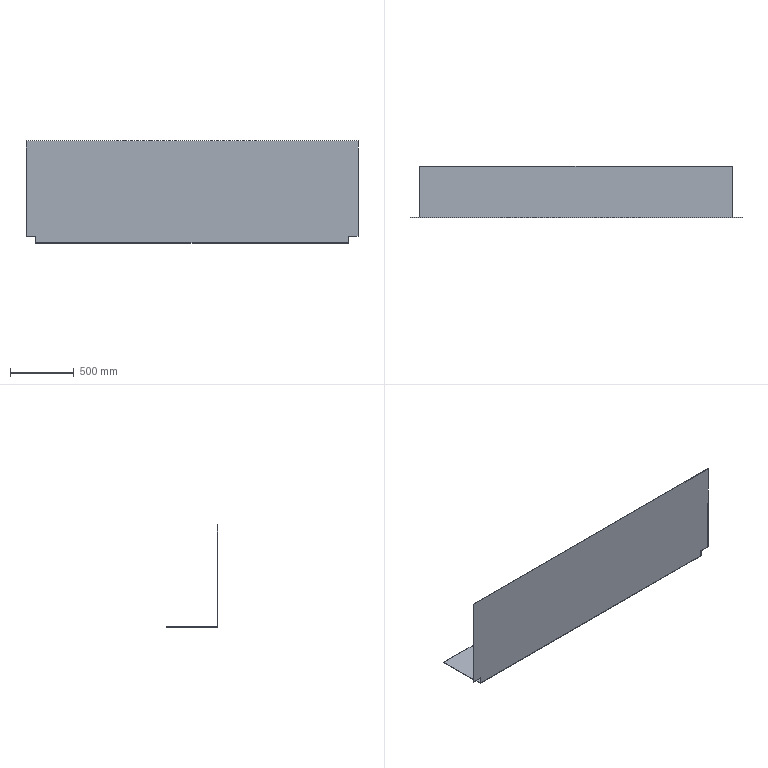Part | STEP file | E3-花纹Plate折弯3 | 1 solid | 14 faces | box 2596 x 403 x 798 mm | volume 9110634 mm3 | plane 12 | cylinder 2 | commonest cylinder face diameters 2 x1 8 x1
STEP:
#1=CARTESIAN_POINT('',(0.,0.,0.));
#2=DIRECTION('',(0.,0.,1.));
#3=DIRECTION('',(1.,0.,0.));
#4=AXIS2_PLACEMENT_3D('',#1,#2,#3);
#5=CARTESIAN_POINT('',(2596.,0.,-746.));
#6=VERTEX_POINT('',#5);
#7=CARTESIAN_POINT('',(2596.,3.,-746.));
#8=VERTEX_POINT('',#7);
#9=CARTESIAN_POINT('',(2596.,3.,-746.));
#10=DIRECTION('',(0.,1.,0.));
#11=VECTOR('',#10,1.);
#12=LINE('',#9,#11);
#13=CARTESIAN_POINT('',(2596.,3.,0.));
#14=DIRECTION('',(1.,0.,0.));
#15=DIRECTION('',(0.,0.,1.));
#16=AXIS2_PLACEMENT_3D('',#13,#14,#15);
#17=PLANE('',#16);
#18=CARTESIAN_POINT('',(-746.,0.));
#19=DIRECTION('',(0.,-1.));
#20=VECTOR('',#19,1.);
#21=LINE('',#18,#20);
#22=(GEOMETRIC_REPRESENTATION_CONTEXT(2)PARAMETRIC_REPRESENTATION_CONTEXT()REPRESENTATION_CONTEXT('',''));
#23=DEFINITIONAL_REPRESENTATION('',(#21),#22);
#24=PCURVE('',#17,#23);
#25=CARTESIAN_POINT('',(2518.,-497.,-746.));
#26=DIRECTION('',(0.,0.,1.));
#27=DIRECTION('',(-1.,0.,0.));
#28=AXIS2_PLACEMENT_3D('',#25,#26,#27);
#29=PLANE('',#28);
#30=CARTESIAN_POINT('',(-78.,-500.));
#31=DIRECTION('',(0.,-1.));
#32=VECTOR('',#31,1.);
#33=LINE('',#30,#32);
#34=(GEOMETRIC_REPRESENTATION_CONTEXT(2)PARAMETRIC_REPRESENTATION_CONTEXT()REPRESENTATION_CONTEXT('',''));
#35=DEFINITIONAL_REPRESENTATION('',(#33),#34);
#36=PCURVE('',#29,#35);
#37=SURFACE_CURVE('',#12,(#24,#36),.PCURVE_S1.);
#38=EDGE_CURVE('',#6,#8,#37,.T.);
#39=ORIENTED_EDGE('',*,*,#38,.T.);
#40=CARTESIAN_POINT('',(2596.,3.,0.));
#41=VERTEX_POINT('',#40);
#42=CARTESIAN_POINT('',(2596.,3.,0.));
#43=DIRECTION('',(0.,0.,1.));
#44=VECTOR('',#43,1.);
#45=LINE('',#42,#44);
#46=CARTESIAN_POINT('',(0.,0.));
#47=DIRECTION('',(1.,0.));
#48=VECTOR('',#47,1.);
#49=LINE('',#46,#48);
#50=(GEOMETRIC_REPRESENTATION_CONTEXT(2)PARAMETRIC_REPRESENTATION_CONTEXT()REPRESENTATION_CONTEXT('',''));
#51=DEFINITIONAL_REPRESENTATION('',(#49),#50);
#52=PCURVE('',#17,#51);
#53=CARTESIAN_POINT('',(0.,3.,0.));
#54=DIRECTION('',(0.,1.,0.));
#55=DIRECTION('',(0.,0.,-1.));
#56=AXIS2_PLACEMENT_3D('',#53,#54,#55);
#57=PLANE('',#56);
#58=CARTESIAN_POINT('',(0.,-2596.));
#59=DIRECTION('',(-1.,0.));
#60=VECTOR('',#59,1.);
#61=LINE('',#58,#60);
#62=(GEOMETRIC_REPRESENTATION_CONTEXT(2)PARAMETRIC_REPRESENTATION_CONTEXT()REPRESENTATION_CONTEXT('',''));
#63=DEFINITIONAL_REPRESENTATION('',(#61),#62);
#64=PCURVE('',#57,#63);
#65=SURFACE_CURVE('',#45,(#52,#64),.PCURVE_S1.);
#66=EDGE_CURVE('',#8,#41,#65,.T.);
#67=ORIENTED_EDGE('',*,*,#66,.T.);
#68=CARTESIAN_POINT('',(2596.,0.,0.));
#69=VERTEX_POINT('',#68);
#70=CARTESIAN_POINT('',(2596.,3.,0.));
#71=DIRECTION('',(0.,1.,0.));
#72=VECTOR('',#71,1.);
#73=LINE('',#70,#72);
#74=CARTESIAN_POINT('',(0.,0.));
#75=DIRECTION('',(0.,-1.));
#76=VECTOR('',#75,1.);
#77=LINE('',#74,#76);
#78=(GEOMETRIC_REPRESENTATION_CONTEXT(2)PARAMETRIC_REPRESENTATION_CONTEXT()REPRESENTATION_CONTEXT('',''));
#79=DEFINITIONAL_REPRESENTATION('',(#77),#78);
#80=PCURVE('',#17,#79);
#81=CARTESIAN_POINT('',(0.,3.,0.));
#82=DIRECTION('',(0.,0.,1.));
#83=DIRECTION('',(-1.,0.,0.));
#84=AXIS2_PLACEMENT_3D('',#81,#82,#83);
#85=PLANE('',#84);
#86=CARTESIAN_POINT('',(-2596.,0.));
#87=DIRECTION('',(0.,-1.));
#88=VECTOR('',#87,1.);
#89=LINE('',#86,#88);
#90=(GEOMETRIC_REPRESENTATION_CONTEXT(2)PARAMETRIC_REPRESENTATION_CONTEXT()REPRESENTATION_CONTEXT('',''));
#91=DEFINITIONAL_REPRESENTATION('',(#89),#90);
#92=PCURVE('',#85,#91);
#93=SURFACE_CURVE('',#73,(#80,#92),.PCURVE_S1.);
#94=EDGE_CURVE('',#69,#41,#93,.T.);
#95=ORIENTED_EDGE('',*,*,#94,.F.);
#96=CARTESIAN_POINT('',(2596.,0.,0.));
#97=DIRECTION('',(0.,0.,1.));
#98=VECTOR('',#97,1.);
#99=LINE('',#96,#98);
#100=CARTESIAN_POINT('',(0.,3.));
#101=DIRECTION('',(1.,0.));
#102=VECTOR('',#101,1.);
#103=LINE('',#100,#102);
#104=(GEOMETRIC_REPRESENTATION_CONTEXT(2)PARAMETRIC_REPRESENTATION_CONTEXT()REPRESENTATION_CONTEXT('',''));
#105=DEFINITIONAL_REPRESENTATION('',(#103),#104);
#106=PCURVE('',#17,#105);
#107=CARTESIAN_POINT('',(0.,0.,0.));
#108=DIRECTION('',(0.,1.,0.));
#109=DIRECTION('',(0.,0.,-1.));
#110=AXIS2_PLACEMENT_3D('',#107,#108,#109);
#111=PLANE('',#110);
#112=CARTESIAN_POINT('',(0.,-2596.));
#113=DIRECTION('',(-1.,0.));
#114=VECTOR('',#113,1.);
#115=LINE('',#112,#114);
#116=(GEOMETRIC_REPRESENTATION_CONTEXT(2)PARAMETRIC_REPRESENTATION_CONTEXT()REPRESENTATION_CONTEXT('',''));
#117=DEFINITIONAL_REPRESENTATION('',(#115),#116);
#118=PCURVE('',#111,#117);
#119=SURFACE_CURVE('',#99,(#106,#118),.PCURVE_S1.);
#120=EDGE_CURVE('',#6,#69,#119,.T.);
#121=ORIENTED_EDGE('',*,*,#120,.F.);
#122=EDGE_LOOP('',(#39,#67,#95,#121));
#123=FACE_BOUND('',#122,.T.);
#124=ADVANCED_FACE('',(#123),#17,.T.);
#125=CARTESIAN_POINT('',(2518.,3.,-746.));
#126=VERTEX_POINT('',#125);
#127=CARTESIAN_POINT('',(2518.,3.,-794.));
#128=VERTEX_POINT('',#127);
#129=CARTESIAN_POINT('',(2518.,3.,0.));
#130=DIRECTION('',(0.,0.,-1.));
#131=VECTOR('',#130,1.);
#132=LINE('',#129,#131);
#133=CARTESIAN_POINT('',(0.,-2518.));
#134=DIRECTION('',(1.,0.));
#135=VECTOR('',#134,1.);
#136=LINE('',#133,#135);
#137=(GEOMETRIC_REPRESENTATION_CONTEXT(2)PARAMETRIC_REPRESENTATION_CONTEXT()REPRESENTATION_CONTEXT('',''));
#138=DEFINITIONAL_REPRESENTATION('',(#136),#137);
#139=PCURVE('',#57,#138);
#140=CARTESIAN_POINT('',(2518.,-497.,-798.));
#141=DIRECTION('',(-1.,0.,0.));
#142=DIRECTION('',(0.,0.,-1.));
#143=AXIS2_PLACEMENT_3D('',#140,#141,#142);
#144=PLANE('',#143);
#145=CARTESIAN_POINT('',(-798.,-500.));
#146=DIRECTION('',(1.,0.));
#147=VECTOR('',#146,1.);
#148=LINE('',#145,#147);
#149=(GEOMETRIC_REPRESENTATION_CONTEXT(2)PARAMETRIC_REPRESENTATION_CONTEXT()REPRESENTATION_CONTEXT('',''));
#150=DEFINITIONAL_REPRESENTATION('',(#148),#149);
#151=PCURVE('',#144,#150);
#152=SURFACE_CURVE('',#132,(#139,#151),.PCURVE_S1.);
#153=EDGE_CURVE('',#126,#128,#152,.T.);
#154=ORIENTED_EDGE('',*,*,#153,.T.);
#155=CARTESIAN_POINT('',(78.,3.,-794.));
#156=VERTEX_POINT('',#155);
#157=CARTESIAN_POINT('',(2596.,3.,-794.));
#158=DIRECTION('',(-1.,0.,0.));
#159=VECTOR('',#158,1.);
#160=LINE('',#157,#159);
#161=CARTESIAN_POINT('',(794.,-2596.));
#162=DIRECTION('',(0.,1.));
#163=VECTOR('',#162,1.);
#164=LINE('',#161,#163);
#165=(GEOMETRIC_REPRESENTATION_CONTEXT(2)PARAMETRIC_REPRESENTATION_CONTEXT()REPRESENTATION_CONTEXT('',''));
#166=DEFINITIONAL_REPRESENTATION('',(#164),#165);
#167=PCURVE('',#57,#166);
#168=CARTESIAN_POINT('',(2596.,4.,-794.));
#169=DIRECTION('',(1.,0.,0.));
#170=DIRECTION('',(0.,0.,-1.));
#171=AXIS2_PLACEMENT_3D('',#168,#169,#170);
#172=CYLINDRICAL_SURFACE('',#171,1.);
#173=CARTESIAN_POINT('',(4.712,0.));
#174=DIRECTION('',(0.,-1.));
#175=VECTOR('',#174,1.);
#176=LINE('',#173,#175);
#177=(GEOMETRIC_REPRESENTATION_CONTEXT(2)PARAMETRIC_REPRESENTATION_CONTEXT()REPRESENTATION_CONTEXT('',''));
#178=DEFINITIONAL_REPRESENTATION('',(#176),#177);
#179=PCURVE('',#172,#178);
#180=SURFACE_CURVE('',#160,(#167,#179),.PCURVE_S1.);
#181=EDGE_CURVE('',#128,#156,#180,.T.);
#182=ORIENTED_EDGE('',*,*,#181,.T.);
#183=CARTESIAN_POINT('',(78.,3.,-746.));
#184=VERTEX_POINT('',#183);
#185=CARTESIAN_POINT('',(78.,3.,0.));
#186=DIRECTION('',(0.,0.,1.));
#187=VECTOR('',#186,1.);
#188=LINE('',#185,#187);
#189=CARTESIAN_POINT('',(0.,-78.));
#190=DIRECTION('',(-1.,0.));
#191=VECTOR('',#190,1.);
#192=LINE('',#189,#191);
#193=(GEOMETRIC_REPRESENTATION_CONTEXT(2)PARAMETRIC_REPRESENTATION_CONTEXT()REPRESENTATION_CONTEXT('',''));
#194=DEFINITIONAL_REPRESENTATION('',(#192),#193);
#195=PCURVE('',#57,#194);
#196=CARTESIAN_POINT('',(78.,-497.,-798.));
#197=DIRECTION('',(1.,0.,0.));
#198=DIRECTION('',(0.,0.,1.));
#199=AXIS2_PLACEMENT_3D('',#196,#197,#198);
#200=PLANE('',#199);
#201=CARTESIAN_POINT('',(798.,-500.));
#202=DIRECTION('',(1.,0.));
#203=VECTOR('',#202,1.);
#204=LINE('',#201,#203);
#205=(GEOMETRIC_REPRESENTATION_CONTEXT(2)PARAMETRIC_REPRESENTATION_CONTEXT()REPRESENTATION_CONTEXT('',''));
#206=DEFINITIONAL_REPRESENTATION('',(#204),#205);
#207=PCURVE('',#200,#206);
#208=SURFACE_CURVE('',#188,(#195,#207),.PCURVE_S1.);
#209=EDGE_CURVE('',#156,#184,#208,.T.);
#210=ORIENTED_EDGE('',*,*,#209,.T.);
#211=CARTESIAN_POINT('',(0.,3.,-746.));
#212=VERTEX_POINT('',#211);
#213=CARTESIAN_POINT('',(0.,3.,-746.));
#214=DIRECTION('',(-1.,0.,0.));
#215=VECTOR('',#214,1.);
#216=LINE('',#213,#215);
#217=CARTESIAN_POINT('',(746.,0.));
#218=DIRECTION('',(0.,1.));
#219=VECTOR('',#218,1.);
#220=LINE('',#217,#219);
#221=(GEOMETRIC_REPRESENTATION_CONTEXT(2)PARAMETRIC_REPRESENTATION_CONTEXT()REPRESENTATION_CONTEXT('',''));
#222=DEFINITIONAL_REPRESENTATION('',(#220),#221);
#223=PCURVE('',#57,#222);
#224=CARTESIAN_POINT('',(-82.,-497.,-746.));
#225=DIRECTION('',(0.,0.,1.));
#226=DIRECTION('',(-1.,0.,0.));
#227=AXIS2_PLACEMENT_3D('',#224,#225,#226);
#228=PLANE('',#227);
#229=CARTESIAN_POINT('',(-82.,-500.));
#230=DIRECTION('',(1.,0.));
#231=VECTOR('',#230,1.);
#232=LINE('',#229,#231);
#233=(GEOMETRIC_REPRESENTATION_CONTEXT(2)PARAMETRIC_REPRESENTATION_CONTEXT()REPRESENTATION_CONTEXT('',''));
#234=DEFINITIONAL_REPRESENTATION('',(#232),#233);
#235=PCURVE('',#228,#234);
#236=SURFACE_CURVE('',#216,(#223,#235),.PCURVE_S1.);
#237=EDGE_CURVE('',#184,#212,#236,.T.);
#238=ORIENTED_EDGE('',*,*,#237,.T.);
#239=CARTESIAN_POINT('',(0.,3.,0.));
#240=VERTEX_POINT('',#239);
#241=CARTESIAN_POINT('',(0.,3.,0.));
#242=DIRECTION('',(0.,0.,-1.));
#243=VECTOR('',#242,1.);
#244=LINE('',#241,#243);
#245=CARTESIAN_POINT('',(0.,0.));
#246=DIRECTION('',(1.,0.));
#247=VECTOR('',#246,1.);
#248=LINE('',#245,#247);
#249=(GEOMETRIC_REPRESENTATION_CONTEXT(2)PARAMETRIC_REPRESENTATION_CONTEXT()REPRESENTATION_CONTEXT('',''));
#250=DEFINITIONAL_REPRESENTATION('',(#248),#249);
#251=PCURVE('',#57,#250);
#252=CARTESIAN_POINT('',(0.,3.,0.));
#253=DIRECTION('',(-1.,0.,0.));
#254=DIRECTION('',(0.,0.,-1.));
#255=AXIS2_PLACEMENT_3D('',#252,#253,#254);
#256=PLANE('',#255);
#257=CARTESIAN_POINT('',(0.,0.));
#258=DIRECTION('',(1.,0.));
#259=VECTOR('',#258,1.);
#260=LINE('',#257,#259);
#261=(GEOMETRIC_REPRESENTATION_CONTEXT(2)PARAMETRIC_REPRESENTATION_CONTEXT()REPRESENTATION_CONTEXT('',''));
#262=DEFINITIONAL_REPRESENTATION('',(#260),#261);
#263=PCURVE('',#256,#262);
#264=SURFACE_CURVE('',#244,(#251,#263),.PCURVE_S1.);
#265=EDGE_CURVE('',#240,#212,#264,.T.);
#266=ORIENTED_EDGE('',*,*,#265,.F.);
#267=CARTESIAN_POINT('',(0.,3.,0.));
#268=DIRECTION('',(-1.,0.,0.));
#269=VECTOR('',#268,1.);
#270=LINE('',#267,#269);
#271=CARTESIAN_POINT('',(0.,0.));
#272=DIRECTION('',(0.,1.));
#273=VECTOR('',#272,1.);
#274=LINE('',#271,#273);
#275=(GEOMETRIC_REPRESENTATION_CONTEXT(2)PARAMETRIC_REPRESENTATION_CONTEXT()REPRESENTATION_CONTEXT('',''));
#276=DEFINITIONAL_REPRESENTATION('',(#274),#275);
#277=PCURVE('',#57,#276);
#278=CARTESIAN_POINT('',(0.,0.));
#279=DIRECTION('',(1.,0.));
#280=VECTOR('',#279,1.);
#281=LINE('',#278,#280);
#282=(GEOMETRIC_REPRESENTATION_CONTEXT(2)PARAMETRIC_REPRESENTATION_CONTEXT()REPRESENTATION_CONTEXT('',''));
#283=DEFINITIONAL_REPRESENTATION('',(#281),#282);
#284=PCURVE('',#85,#283);
#285=SURFACE_CURVE('',#270,(#277,#284),.PCURVE_S1.);
#286=EDGE_CURVE('',#41,#240,#285,.T.);
#287=ORIENTED_EDGE('',*,*,#286,.F.);
#288=ORIENTED_EDGE('',*,*,#66,.F.);
#289=CARTESIAN_POINT('',(0.,3.,-746.));
#290=DIRECTION('',(-1.,0.,0.));
#291=VECTOR('',#290,1.);
#292=LINE('',#289,#291);
#293=CARTESIAN_POINT('',(746.,0.));
#294=DIRECTION('',(0.,1.));
#295=VECTOR('',#294,1.);
#296=LINE('',#293,#295);
#297=(GEOMETRIC_REPRESENTATION_CONTEXT(2)PARAMETRIC_REPRESENTATION_CONTEXT()REPRESENTATION_CONTEXT('',''));
#298=DEFINITIONAL_REPRESENTATION('',(#296),#297);
#299=PCURVE('',#57,#298);
#300=CARTESIAN_POINT('',(2518.,-500.));
#301=DIRECTION('',(1.,0.));
#302=VECTOR('',#301,1.);
#303=LINE('',#300,#302);
#304=(GEOMETRIC_REPRESENTATION_CONTEXT(2)PARAMETRIC_REPRESENTATION_CONTEXT()REPRESENTATION_CONTEXT('',''));
#305=DEFINITIONAL_REPRESENTATION('',(#303),#304);
#306=PCURVE('',#29,#305);
#307=SURFACE_CURVE('',#292,(#299,#306),.PCURVE_S1.);
#308=EDGE_CURVE('',#8,#126,#307,.T.);
#309=ORIENTED_EDGE('',*,*,#308,.T.);
#310=EDGE_LOOP('',(#154,#182,#210,#238,#266,#287,#288,#309));
#311=FACE_BOUND('',#310,.T.);
#312=ADVANCED_FACE('',(#311),#57,.T.);
#313=CARTESIAN_POINT('',(2518.,0.,-746.));
#314=VERTEX_POINT('',#313);
#315=CARTESIAN_POINT('',(0.,0.,-746.));
#316=DIRECTION('',(-1.,0.,0.));
#317=VECTOR('',#316,1.);
#318=LINE('',#315,#317);
#319=CARTESIAN_POINT('',(746.,0.));
#320=DIRECTION('',(0.,1.));
#321=VECTOR('',#320,1.);
#322=LINE('',#319,#321);
#323=(GEOMETRIC_REPRESENTATION_CONTEXT(2)PARAMETRIC_REPRESENTATION_CONTEXT()REPRESENTATION_CONTEXT('',''));
#324=DEFINITIONAL_REPRESENTATION('',(#322),#323);
#325=PCURVE('',#111,#324);
#326=CARTESIAN_POINT('',(2518.,-497.));
#327=DIRECTION('',(1.,0.));
#328=VECTOR('',#327,1.);
#329=LINE('',#326,#328);
#330=(GEOMETRIC_REPRESENTATION_CONTEXT(2)PARAMETRIC_REPRESENTATION_CONTEXT()REPRESENTATION_CONTEXT('',''));
#331=DEFINITIONAL_REPRESENTATION('',(#329),#330);
#332=PCURVE('',#29,#331);
#333=SURFACE_CURVE('',#318,(#325,#332),.PCURVE_S1.);
#334=EDGE_CURVE('',#6,#314,#333,.T.);
#335=ORIENTED_EDGE('',*,*,#334,.F.);
#336=ORIENTED_EDGE('',*,*,#120,.T.);
#337=CARTESIAN_POINT('',(0.,0.,0.));
#338=VERTEX_POINT('',#337);
#339=CARTESIAN_POINT('',(0.,0.,0.));
#340=DIRECTION('',(-1.,0.,0.));
#341=VECTOR('',#340,1.);
#342=LINE('',#339,#341);
#343=CARTESIAN_POINT('',(0.,0.));
#344=DIRECTION('',(0.,1.));
#345=VECTOR('',#344,1.);
#346=LINE('',#343,#345);
#347=(GEOMETRIC_REPRESENTATION_CONTEXT(2)PARAMETRIC_REPRESENTATION_CONTEXT()REPRESENTATION_CONTEXT('',''));
#348=DEFINITIONAL_REPRESENTATION('',(#346),#347);
#349=PCURVE('',#111,#348);
#350=CARTESIAN_POINT('',(0.,3.));
#351=DIRECTION('',(1.,0.));
#352=VECTOR('',#351,1.);
#353=LINE('',#350,#352);
#354=(GEOMETRIC_REPRESENTATION_CONTEXT(2)PARAMETRIC_REPRESENTATION_CONTEXT()REPRESENTATION_CONTEXT('',''));
#355=DEFINITIONAL_REPRESENTATION('',(#353),#354);
#356=PCURVE('',#85,#355);
#357=SURFACE_CURVE('',#342,(#349,#356),.PCURVE_S1.);
#358=EDGE_CURVE('',#69,#338,#357,.T.);
#359=ORIENTED_EDGE('',*,*,#358,.T.);
#360=CARTESIAN_POINT('',(0.,0.,-746.));
#361=VERTEX_POINT('',#360);
#362=CARTESIAN_POINT('',(0.,0.,0.));
#363=DIRECTION('',(0.,0.,-1.));
#364=VECTOR('',#363,1.);
#365=LINE('',#362,#364);
#366=CARTESIAN_POINT('',(0.,0.));
#367=DIRECTION('',(1.,0.));
#368=VECTOR('',#367,1.);
#369=LINE('',#366,#368);
#370=(GEOMETRIC_REPRESENTATION_CONTEXT(2)PARAMETRIC_REPRESENTATION_CONTEXT()REPRESENTATION_CONTEXT('',''));
#371=DEFINITIONAL_REPRESENTATION('',(#369),#370);
#372=PCURVE('',#111,#371);
#373=CARTESIAN_POINT('',(0.,3.));
#374=DIRECTION('',(1.,0.));
#375=VECTOR('',#374,1.);
#376=LINE('',#373,#375);
#377=(GEOMETRIC_REPRESENTATION_CONTEXT(2)PARAMETRIC_REPRESENTATION_CONTEXT()REPRESENTATION_CONTEXT('',''));
#378=DEFINITIONAL_REPRESENTATION('',(#376),#377);
#379=PCURVE('',#256,#378);
#380=SURFACE_CURVE('',#365,(#372,#379),.PCURVE_S1.);
#381=EDGE_CURVE('',#338,#361,#380,.T.);
#382=ORIENTED_EDGE('',*,*,#381,.T.);
#383=CARTESIAN_POINT('',(78.,0.,-746.));
#384=VERTEX_POINT('',#383);
#385=CARTESIAN_POINT('',(0.,0.,-746.));
#386=DIRECTION('',(-1.,0.,0.));
#387=VECTOR('',#386,1.);
#388=LINE('',#385,#387);
#389=CARTESIAN_POINT('',(746.,0.));
#390=DIRECTION('',(0.,1.));
#391=VECTOR('',#390,1.);
#392=LINE('',#389,#391);
#393=(GEOMETRIC_REPRESENTATION_CONTEXT(2)PARAMETRIC_REPRESENTATION_CONTEXT()REPRESENTATION_CONTEXT('',''));
#394=DEFINITIONAL_REPRESENTATION('',(#392),#393);
#395=PCURVE('',#111,#394);
#396=CARTESIAN_POINT('',(-82.,-497.));
#397=DIRECTION('',(1.,0.));
#398=VECTOR('',#397,1.);
#399=LINE('',#396,#398);
#400=(GEOMETRIC_REPRESENTATION_CONTEXT(2)PARAMETRIC_REPRESENTATION_CONTEXT()REPRESENTATION_CONTEXT('',''));
#401=DEFINITIONAL_REPRESENTATION('',(#399),#400);
#402=PCURVE('',#228,#401);
#403=SURFACE_CURVE('',#388,(#395,#402),.PCURVE_S1.);
#404=EDGE_CURVE('',#384,#361,#403,.T.);
#405=ORIENTED_EDGE('',*,*,#404,.F.);
#406=CARTESIAN_POINT('',(78.,0.,-794.));
#407=VERTEX_POINT('',#406);
#408=CARTESIAN_POINT('',(78.,0.,0.));
#409=DIRECTION('',(0.,0.,1.));
#410=VECTOR('',#409,1.);
#411=LINE('',#408,#410);
#412=CARTESIAN_POINT('',(0.,-78.));
#413=DIRECTION('',(-1.,0.));
#414=VECTOR('',#413,1.);
#415=LINE('',#412,#414);
#416=(GEOMETRIC_REPRESENTATION_CONTEXT(2)PARAMETRIC_REPRESENTATION_CONTEXT()REPRESENTATION_CONTEXT('',''));
#417=DEFINITIONAL_REPRESENTATION('',(#415),#416);
#418=PCURVE('',#111,#417);
#419=CARTESIAN_POINT('',(798.,-497.));
#420=DIRECTION('',(1.,0.));
#421=VECTOR('',#420,1.);
#422=LINE('',#419,#421);
#423=(GEOMETRIC_REPRESENTATION_CONTEXT(2)PARAMETRIC_REPRESENTATION_CONTEXT()REPRESENTATION_CONTEXT('',''));
#424=DEFINITIONAL_REPRESENTATION('',(#422),#423);
#425=PCURVE('',#200,#424);
#426=SURFACE_CURVE('',#411,(#418,#425),.PCURVE_S1.);
#427=EDGE_CURVE('',#407,#384,#426,.T.);
#428=ORIENTED_EDGE('',*,*,#427,.F.);
#429=CARTESIAN_POINT('',(2518.,0.,-794.));
#430=VERTEX_POINT('',#429);
#431=CARTESIAN_POINT('',(2596.,0.,-794.));
#432=DIRECTION('',(-1.,0.,0.));
#433=VECTOR('',#432,1.);
#434=LINE('',#431,#433);
#435=CARTESIAN_POINT('',(794.,-2596.));
#436=DIRECTION('',(0.,1.));
#437=VECTOR('',#436,1.);
#438=LINE('',#435,#437);
#439=(GEOMETRIC_REPRESENTATION_CONTEXT(2)PARAMETRIC_REPRESENTATION_CONTEXT()REPRESENTATION_CONTEXT('',''));
#440=DEFINITIONAL_REPRESENTATION('',(#438),#439);
#441=PCURVE('',#111,#440);
#442=CARTESIAN_POINT('',(2596.,4.,-794.));
#443=DIRECTION('',(1.,0.,0.));
#444=DIRECTION('',(0.,0.,-1.));
#445=AXIS2_PLACEMENT_3D('',#442,#443,#444);
#446=CYLINDRICAL_SURFACE('',#445,4.);
#447=CARTESIAN_POINT('',(4.712,0.));
#448=DIRECTION('',(0.,-1.));
#449=VECTOR('',#448,1.);
#450=LINE('',#447,#449);
#451=(GEOMETRIC_REPRESENTATION_CONTEXT(2)PARAMETRIC_REPRESENTATION_CONTEXT()REPRESENTATION_CONTEXT('',''));
#452=DEFINITIONAL_REPRESENTATION('',(#450),#451);
#453=PCURVE('',#446,#452);
#454=SURFACE_CURVE('',#434,(#441,#453),.PCURVE_S1.);
#455=EDGE_CURVE('',#430,#407,#454,.T.);
#456=ORIENTED_EDGE('',*,*,#455,.F.);
#457=CARTESIAN_POINT('',(2518.,0.,0.));
#458=DIRECTION('',(0.,0.,-1.));
#459=VECTOR('',#458,1.);
#460=LINE('',#457,#459);
#461=CARTESIAN_POINT('',(0.,-2518.));
#462=DIRECTION('',(1.,0.));
#463=VECTOR('',#462,1.);
#464=LINE('',#461,#463);
#465=(GEOMETRIC_REPRESENTATION_CONTEXT(2)PARAMETRIC_REPRESENTATION_CONTEXT()REPRESENTATION_CONTEXT('',''));
#466=DEFINITIONAL_REPRESENTATION('',(#464),#465);
#467=PCURVE('',#111,#466);
#468=CARTESIAN_POINT('',(-798.,-497.));
#469=DIRECTION('',(1.,0.));
#470=VECTOR('',#469,1.);
#471=LINE('',#468,#470);
#472=(GEOMETRIC_REPRESENTATION_CONTEXT(2)PARAMETRIC_REPRESENTATION_CONTEXT()REPRESENTATION_CONTEXT('',''));
#473=DEFINITIONAL_REPRESENTATION('',(#471),#472);
#474=PCURVE('',#144,#473);
#475=SURFACE_CURVE('',#460,(#467,#474),.PCURVE_S1.);
#476=EDGE_CURVE('',#314,#430,#475,.T.);
#477=ORIENTED_EDGE('',*,*,#476,.F.);
#478=EDGE_LOOP('',(#335,#336,#359,#382,#405,#428,#456,#477));
#479=FACE_BOUND('',#478,.T.);
#480=ADVANCED_FACE('',(#479),#111,.F.);
#481=ORIENTED_EDGE('',*,*,#94,.T.);
#482=ORIENTED_EDGE('',*,*,#286,.T.);
#483=CARTESIAN_POINT('',(0.,3.,0.));
#484=DIRECTION('',(0.,1.,0.));
#485=VECTOR('',#484,1.);
#486=LINE('',#483,#485);
#487=CARTESIAN_POINT('',(0.,0.));
#488=DIRECTION('',(0.,-1.));
#489=VECTOR('',#488,1.);
#490=LINE('',#487,#489);
#491=(GEOMETRIC_REPRESENTATION_CONTEXT(2)PARAMETRIC_REPRESENTATION_CONTEXT()REPRESENTATION_CONTEXT('',''));
#492=DEFINITIONAL_REPRESENTATION('',(#490),#491);
#493=PCURVE('',#85,#492);
#494=CARTESIAN_POINT('',(0.,0.));
#495=DIRECTION('',(0.,-1.));
#496=VECTOR('',#495,1.);
#497=LINE('',#494,#496);
#498=(GEOMETRIC_REPRESENTATION_CONTEXT(2)PARAMETRIC_REPRESENTATION_CONTEXT()REPRESENTATION_CONTEXT('',''));
#499=DEFINITIONAL_REPRESENTATION('',(#497),#498);
#500=PCURVE('',#256,#499);
#501=SURFACE_CURVE('',#486,(#493,#500),.PCURVE_S1.);
#502=EDGE_CURVE('',#338,#240,#501,.T.);
#503=ORIENTED_EDGE('',*,*,#502,.F.);
#504=ORIENTED_EDGE('',*,*,#358,.F.);
#505=EDGE_LOOP('',(#481,#482,#503,#504));
#506=FACE_BOUND('',#505,.T.);
#507=ADVANCED_FACE('',(#506),#85,.T.);
#508=CARTESIAN_POINT('',(0.,3.,-746.));
#509=DIRECTION('',(0.,-1.,0.));
#510=VECTOR('',#509,1.);
#511=LINE('',#508,#510);
#512=CARTESIAN_POINT('',(746.,0.));
#513=DIRECTION('',(0.,1.));
#514=VECTOR('',#513,1.);
#515=LINE('',#512,#514);
#516=(GEOMETRIC_REPRESENTATION_CONTEXT(2)PARAMETRIC_REPRESENTATION_CONTEXT()REPRESENTATION_CONTEXT('',''));
#517=DEFINITIONAL_REPRESENTATION('',(#515),#516);
#518=PCURVE('',#256,#517);
#519=CARTESIAN_POINT('',(-82.,-500.));
#520=DIRECTION('',(0.,1.));
#521=VECTOR('',#520,1.);
#522=LINE('',#519,#521);
#523=(GEOMETRIC_REPRESENTATION_CONTEXT(2)PARAMETRIC_REPRESENTATION_CONTEXT()REPRESENTATION_CONTEXT('',''));
#524=DEFINITIONAL_REPRESENTATION('',(#522),#523);
#525=PCURVE('',#228,#524);
#526=SURFACE_CURVE('',#511,(#518,#525),.PCURVE_S1.);
#527=EDGE_CURVE('',#212,#361,#526,.T.);
#528=ORIENTED_EDGE('',*,*,#527,.T.);
#529=ORIENTED_EDGE('',*,*,#381,.F.);
#530=ORIENTED_EDGE('',*,*,#502,.T.);
#531=ORIENTED_EDGE('',*,*,#265,.T.);
#532=EDGE_LOOP('',(#528,#529,#530,#531));
#533=FACE_BOUND('',#532,.T.);
#534=ADVANCED_FACE('',(#533),#256,.T.);
#535=CARTESIAN_POINT('',(2518.,4.,-798.));
#536=VERTEX_POINT('',#535);
#537=CARTESIAN_POINT('',(2518.,4.,-794.));
#538=DIRECTION('',(-1.,0.,0.));
#539=DIRECTION('',(0.,0.,-1.));
#540=AXIS2_PLACEMENT_3D('',#537,#538,#539);
#541=CIRCLE('',#540,4.);
#542=CARTESIAN_POINT('',(6.283,-78.));
#543=DIRECTION('',(-1.,0.));
#544=VECTOR('',#543,1.);
#545=LINE('',#542,#544);
#546=(GEOMETRIC_REPRESENTATION_CONTEXT(2)PARAMETRIC_REPRESENTATION_CONTEXT()REPRESENTATION_CONTEXT('',''));
#547=DEFINITIONAL_REPRESENTATION('',(#545),#546);
#548=PCURVE('',#446,#547);
#549=CARTESIAN_POINT('',(-4.,-501.));
#550=DIRECTION('',(1.,0.));
#551=AXIS2_PLACEMENT_2D('',#549,#550);
#552=CIRCLE('',#551,4.);
#553=(GEOMETRIC_REPRESENTATION_CONTEXT(2)PARAMETRIC_REPRESENTATION_CONTEXT()REPRESENTATION_CONTEXT('',''));
#554=DEFINITIONAL_REPRESENTATION('',(#552),#553);
#555=PCURVE('',#144,#554);
#556=SURFACE_CURVE('',#541,(#548,#555),.PCURVE_S1.);
#557=EDGE_CURVE('',#536,#430,#556,.T.);
#558=ORIENTED_EDGE('',*,*,#557,.T.);
#559=ORIENTED_EDGE('',*,*,#455,.T.);
#560=CARTESIAN_POINT('',(78.,4.,-798.));
#561=VERTEX_POINT('',#560);
#562=CARTESIAN_POINT('',(78.,4.,-794.));
#563=DIRECTION('',(1.,0.,0.));
#564=DIRECTION('',(0.,0.,1.));
#565=AXIS2_PLACEMENT_3D('',#562,#563,#564);
#566=CIRCLE('',#565,4.);
#567=CARTESIAN_POINT('',(3.142,-2518.));
#568=DIRECTION('',(1.,0.));
#569=VECTOR('',#568,1.);
#570=LINE('',#567,#569);
#571=(GEOMETRIC_REPRESENTATION_CONTEXT(2)PARAMETRIC_REPRESENTATION_CONTEXT()REPRESENTATION_CONTEXT('',''));
#572=DEFINITIONAL_REPRESENTATION('',(#570),#571);
#573=PCURVE('',#446,#572);
#574=CARTESIAN_POINT('',(4.,-501.));
#575=DIRECTION('',(1.,0.));
#576=AXIS2_PLACEMENT_2D('',#574,#575);
#577=CIRCLE('',#576,4.);
#578=(GEOMETRIC_REPRESENTATION_CONTEXT(2)PARAMETRIC_REPRESENTATION_CONTEXT()REPRESENTATION_CONTEXT('',''));
#579=DEFINITIONAL_REPRESENTATION('',(#577),#578);
#580=PCURVE('',#200,#579);
#581=SURFACE_CURVE('',#566,(#573,#580),.PCURVE_S1.);
#582=EDGE_CURVE('',#407,#561,#581,.T.);
#583=ORIENTED_EDGE('',*,*,#582,.T.);
#584=CARTESIAN_POINT('',(0.,4.,-798.));
#585=DIRECTION('',(-1.,0.,0.));
#586=VECTOR('',#585,1.);
#587=LINE('',#584,#586);
#588=CARTESIAN_POINT('',(6.283,-2596.));
#589=DIRECTION('',(0.,-1.));
#590=VECTOR('',#589,1.);
#591=LINE('',#588,#590);
#592=(GEOMETRIC_REPRESENTATION_CONTEXT(2)PARAMETRIC_REPRESENTATION_CONTEXT()REPRESENTATION_CONTEXT('',''));
#593=DEFINITIONAL_REPRESENTATION('',(#591),#592);
#594=PCURVE('',#446,#593);
#595=CARTESIAN_POINT('',(0.,0.,-798.));
#596=DIRECTION('',(0.,0.,1.));
#597=DIRECTION('',(-1.,0.,0.));
#598=AXIS2_PLACEMENT_3D('',#595,#596,#597);
#599=PLANE('',#598);
#600=CARTESIAN_POINT('',(0.,-4.));
#601=DIRECTION('',(1.,0.));
#602=VECTOR('',#601,1.);
#603=LINE('',#600,#602);
#604=(GEOMETRIC_REPRESENTATION_CONTEXT(2)PARAMETRIC_REPRESENTATION_CONTEXT()REPRESENTATION_CONTEXT('',''));
#605=DEFINITIONAL_REPRESENTATION('',(#603),#604);
#606=PCURVE('',#599,#605);
#607=SURFACE_CURVE('',#587,(#594,#606),.PCURVE_S1.);
#608=EDGE_CURVE('',#536,#561,#607,.T.);
#609=ORIENTED_EDGE('',*,*,#608,.F.);
#610=EDGE_LOOP('',(#558,#559,#583,#609));
#611=FACE_BOUND('',#610,.T.);
#612=ADVANCED_FACE('',(#611),#446,.T.);
#613=CARTESIAN_POINT('',(2518.,4.,-795.));
#614=VERTEX_POINT('',#613);
#615=CARTESIAN_POINT('',(2518.,4.,-794.));
#616=DIRECTION('',(-1.,0.,0.));
#617=DIRECTION('',(0.,0.,-1.));
#618=AXIS2_PLACEMENT_3D('',#615,#616,#617);
#619=CIRCLE('',#618,1.);
#620=CARTESIAN_POINT('',(6.283,-78.));
#621=DIRECTION('',(-1.,0.));
#622=VECTOR('',#621,1.);
#623=LINE('',#620,#622);
#624=(GEOMETRIC_REPRESENTATION_CONTEXT(2)PARAMETRIC_REPRESENTATION_CONTEXT()REPRESENTATION_CONTEXT('',''));
#625=DEFINITIONAL_REPRESENTATION('',(#623),#624);
#626=PCURVE('',#172,#625);
#627=CARTESIAN_POINT('',(-4.,-501.));
#628=DIRECTION('',(1.,0.));
#629=AXIS2_PLACEMENT_2D('',#627,#628);
#630=CIRCLE('',#629,1.);
#631=(GEOMETRIC_REPRESENTATION_CONTEXT(2)PARAMETRIC_REPRESENTATION_CONTEXT()REPRESENTATION_CONTEXT('',''));
#632=DEFINITIONAL_REPRESENTATION('',(#630),#631);
#633=PCURVE('',#144,#632);
#634=SURFACE_CURVE('',#619,(#626,#633),.PCURVE_S1.);
#635=EDGE_CURVE('',#614,#128,#634,.T.);
#636=ORIENTED_EDGE('',*,*,#635,.T.);
#637=ORIENTED_EDGE('',*,*,#181,.T.);
#638=CARTESIAN_POINT('',(78.,4.,-795.));
#639=VERTEX_POINT('',#638);
#640=CARTESIAN_POINT('',(78.,4.,-794.));
#641=DIRECTION('',(1.,0.,0.));
#642=DIRECTION('',(0.,0.,1.));
#643=AXIS2_PLACEMENT_3D('',#640,#641,#642);
#644=CIRCLE('',#643,1.);
#645=CARTESIAN_POINT('',(3.142,-2518.));
#646=DIRECTION('',(1.,0.));
#647=VECTOR('',#646,1.);
#648=LINE('',#645,#647);
#649=(GEOMETRIC_REPRESENTATION_CONTEXT(2)PARAMETRIC_REPRESENTATION_CONTEXT()REPRESENTATION_CONTEXT('',''));
#650=DEFINITIONAL_REPRESENTATION('',(#648),#649);
#651=PCURVE('',#172,#650);
#652=CARTESIAN_POINT('',(4.,-501.));
#653=DIRECTION('',(1.,0.));
#654=AXIS2_PLACEMENT_2D('',#652,#653);
#655=CIRCLE('',#654,1.);
#656=(GEOMETRIC_REPRESENTATION_CONTEXT(2)PARAMETRIC_REPRESENTATION_CONTEXT()REPRESENTATION_CONTEXT('',''));
#657=DEFINITIONAL_REPRESENTATION('',(#655),#656);
#658=PCURVE('',#200,#657);
#659=SURFACE_CURVE('',#644,(#651,#658),.PCURVE_S1.);
#660=EDGE_CURVE('',#156,#639,#659,.T.);
#661=ORIENTED_EDGE('',*,*,#660,.T.);
#662=CARTESIAN_POINT('',(0.,4.,-795.));
#663=DIRECTION('',(1.,0.,0.));
#664=VECTOR('',#663,1.);
#665=LINE('',#662,#664);
#666=CARTESIAN_POINT('',(6.283,-2596.));
#667=DIRECTION('',(0.,1.));
#668=VECTOR('',#667,1.);
#669=LINE('',#666,#668);
#670=(GEOMETRIC_REPRESENTATION_CONTEXT(2)PARAMETRIC_REPRESENTATION_CONTEXT()REPRESENTATION_CONTEXT('',''));
#671=DEFINITIONAL_REPRESENTATION('',(#669),#670);
#672=PCURVE('',#172,#671);
#673=CARTESIAN_POINT('',(0.,0.,-795.));
#674=DIRECTION('',(0.,0.,1.));
#675=DIRECTION('',(-1.,0.,0.));
#676=AXIS2_PLACEMENT_3D('',#673,#674,#675);
#677=PLANE('',#676);
#678=CARTESIAN_POINT('',(0.,-4.));
#679=DIRECTION('',(-1.,0.));
#680=VECTOR('',#679,1.);
#681=LINE('',#678,#680);
#682=(GEOMETRIC_REPRESENTATION_CONTEXT(2)PARAMETRIC_REPRESENTATION_CONTEXT()REPRESENTATION_CONTEXT('',''));
#683=DEFINITIONAL_REPRESENTATION('',(#681),#682);
#684=PCURVE('',#677,#683);
#685=SURFACE_CURVE('',#665,(#672,#684),.PCURVE_S1.);
#686=EDGE_CURVE('',#639,#614,#685,.T.);
#687=ORIENTED_EDGE('',*,*,#686,.T.);
#688=EDGE_LOOP('',(#636,#637,#661,#687));
#689=FACE_BOUND('',#688,.F.);
#690=ADVANCED_FACE('',(#689),#172,.F.);
#691=ORIENTED_EDGE('',*,*,#608,.T.);
#692=CARTESIAN_POINT('',(78.,403.,-798.));
#693=VERTEX_POINT('',#692);
#694=CARTESIAN_POINT('',(78.,-497.,-798.));
#695=DIRECTION('',(0.,1.,0.));
#696=VECTOR('',#695,1.);
#697=LINE('',#694,#696);
#698=CARTESIAN_POINT('',(-78.,497.));
#699=DIRECTION('',(0.,-1.));
#700=VECTOR('',#699,1.);
#701=LINE('',#698,#700);
#702=(GEOMETRIC_REPRESENTATION_CONTEXT(2)PARAMETRIC_REPRESENTATION_CONTEXT()REPRESENTATION_CONTEXT('',''));
#703=DEFINITIONAL_REPRESENTATION('',(#701),#702);
#704=PCURVE('',#599,#703);
#705=CARTESIAN_POINT('',(0.,0.));
#706=DIRECTION('',(0.,-1.));
#707=VECTOR('',#706,1.);
#708=LINE('',#705,#707);
#709=(GEOMETRIC_REPRESENTATION_CONTEXT(2)PARAMETRIC_REPRESENTATION_CONTEXT()REPRESENTATION_CONTEXT('',''));
#710=DEFINITIONAL_REPRESENTATION('',(#708),#709);
#711=PCURVE('',#200,#710);
#712=SURFACE_CURVE('',#697,(#704,#711),.PCURVE_S1.);
#713=EDGE_CURVE('',#561,#693,#712,.T.);
#714=ORIENTED_EDGE('',*,*,#713,.T.);
#715=CARTESIAN_POINT('',(2518.,403.,-798.));
#716=VERTEX_POINT('',#715);
#717=CARTESIAN_POINT('',(0.,403.,-798.));
#718=DIRECTION('',(-1.,0.,0.));
#719=VECTOR('',#718,1.);
#720=LINE('',#717,#719);
#721=CARTESIAN_POINT('',(0.,-403.));
#722=DIRECTION('',(1.,0.));
#723=VECTOR('',#722,1.);
#724=LINE('',#721,#723);
#725=(GEOMETRIC_REPRESENTATION_CONTEXT(2)PARAMETRIC_REPRESENTATION_CONTEXT()REPRESENTATION_CONTEXT('',''));
#726=DEFINITIONAL_REPRESENTATION('',(#724),#725);
#727=PCURVE('',#599,#726);
#728=CARTESIAN_POINT('',(0.,403.,-798.));
#729=DIRECTION('',(0.,-1.,0.));
#730=DIRECTION('',(0.,0.,1.));
#731=AXIS2_PLACEMENT_3D('',#728,#729,#730);
#732=PLANE('',#731);
#733=CARTESIAN_POINT('',(0.,0.));
#734=DIRECTION('',(0.,1.));
#735=VECTOR('',#734,1.);
#736=LINE('',#733,#735);
#737=(GEOMETRIC_REPRESENTATION_CONTEXT(2)PARAMETRIC_REPRESENTATION_CONTEXT()REPRESENTATION_CONTEXT('',''));
#738=DEFINITIONAL_REPRESENTATION('',(#736),#737);
#739=PCURVE('',#732,#738);
#740=SURFACE_CURVE('',#720,(#727,#739),.PCURVE_S1.);
#741=EDGE_CURVE('',#716,#693,#740,.T.);
#742=ORIENTED_EDGE('',*,*,#741,.F.);
#743=CARTESIAN_POINT('',(2518.,-497.,-798.));
#744=DIRECTION('',(0.,1.,0.));
#745=VECTOR('',#744,1.);
#746=LINE('',#743,#745);
#747=CARTESIAN_POINT('',(-2518.,497.));
#748=DIRECTION('',(0.,-1.));
#749=VECTOR('',#748,1.);
#750=LINE('',#747,#749);
#751=(GEOMETRIC_REPRESENTATION_CONTEXT(2)PARAMETRIC_REPRESENTATION_CONTEXT()REPRESENTATION_CONTEXT('',''));
#752=DEFINITIONAL_REPRESENTATION('',(#750),#751);
#753=PCURVE('',#599,#752);
#754=CARTESIAN_POINT('',(0.,0.));
#755=DIRECTION('',(0.,-1.));
#756=VECTOR('',#755,1.);
#757=LINE('',#754,#756);
#758=(GEOMETRIC_REPRESENTATION_CONTEXT(2)PARAMETRIC_REPRESENTATION_CONTEXT()REPRESENTATION_CONTEXT('',''));
#759=DEFINITIONAL_REPRESENTATION('',(#757),#758);
#760=PCURVE('',#144,#759);
#761=SURFACE_CURVE('',#746,(#753,#760),.PCURVE_S1.);
#762=EDGE_CURVE('',#536,#716,#761,.T.);
#763=ORIENTED_EDGE('',*,*,#762,.F.);
#764=EDGE_LOOP('',(#691,#714,#742,#763));
#765=FACE_BOUND('',#764,.T.);
#766=ADVANCED_FACE('',(#765),#599,.F.);
#767=CARTESIAN_POINT('',(2518.,403.,-795.));
#768=VERTEX_POINT('',#767);
#769=CARTESIAN_POINT('',(2518.,0.,-795.));
#770=DIRECTION('',(0.,1.,0.));
#771=VECTOR('',#770,1.);
#772=LINE('',#769,#771);
#773=CARTESIAN_POINT('',(-2518.,0.));
#774=DIRECTION('',(0.,-1.));
#775=VECTOR('',#774,1.);
#776=LINE('',#773,#775);
#777=(GEOMETRIC_REPRESENTATION_CONTEXT(2)PARAMETRIC_REPRESENTATION_CONTEXT()REPRESENTATION_CONTEXT('',''));
#778=DEFINITIONAL_REPRESENTATION('',(#776),#777);
#779=PCURVE('',#677,#778);
#780=CARTESIAN_POINT('',(-3.,-497.));
#781=DIRECTION('',(0.,-1.));
#782=VECTOR('',#781,1.);
#783=LINE('',#780,#782);
#784=(GEOMETRIC_REPRESENTATION_CONTEXT(2)PARAMETRIC_REPRESENTATION_CONTEXT()REPRESENTATION_CONTEXT('',''));
#785=DEFINITIONAL_REPRESENTATION('',(#783),#784);
#786=PCURVE('',#144,#785);
#787=SURFACE_CURVE('',#772,(#779,#786),.PCURVE_S1.);
#788=EDGE_CURVE('',#614,#768,#787,.T.);
#789=ORIENTED_EDGE('',*,*,#788,.T.);
#790=CARTESIAN_POINT('',(78.,403.,-795.));
#791=VERTEX_POINT('',#790);
#792=CARTESIAN_POINT('',(0.,403.,-795.));
#793=DIRECTION('',(-1.,0.,0.));
#794=VECTOR('',#793,1.);
#795=LINE('',#792,#794);
#796=CARTESIAN_POINT('',(0.,-403.));
#797=DIRECTION('',(1.,0.));
#798=VECTOR('',#797,1.);
#799=LINE('',#796,#798);
#800=(GEOMETRIC_REPRESENTATION_CONTEXT(2)PARAMETRIC_REPRESENTATION_CONTEXT()REPRESENTATION_CONTEXT('',''));
#801=DEFINITIONAL_REPRESENTATION('',(#799),#800);
#802=PCURVE('',#677,#801);
#803=CARTESIAN_POINT('',(3.,0.));
#804=DIRECTION('',(0.,1.));
#805=VECTOR('',#804,1.);
#806=LINE('',#803,#805);
#807=(GEOMETRIC_REPRESENTATION_CONTEXT(2)PARAMETRIC_REPRESENTATION_CONTEXT()REPRESENTATION_CONTEXT('',''));
#808=DEFINITIONAL_REPRESENTATION('',(#806),#807);
#809=PCURVE('',#732,#808);
#810=SURFACE_CURVE('',#795,(#802,#809),.PCURVE_S1.);
#811=EDGE_CURVE('',#768,#791,#810,.T.);
#812=ORIENTED_EDGE('',*,*,#811,.T.);
#813=CARTESIAN_POINT('',(78.,0.,-795.));
#814=DIRECTION('',(0.,-1.,0.));
#815=VECTOR('',#814,1.);
#816=LINE('',#813,#815);
#817=CARTESIAN_POINT('',(-78.,0.));
#818=DIRECTION('',(0.,1.));
#819=VECTOR('',#818,1.);
#820=LINE('',#817,#819);
#821=(GEOMETRIC_REPRESENTATION_CONTEXT(2)PARAMETRIC_REPRESENTATION_CONTEXT()REPRESENTATION_CONTEXT('',''));
#822=DEFINITIONAL_REPRESENTATION('',(#820),#821);
#823=PCURVE('',#677,#822);
#824=CARTESIAN_POINT('',(3.,-497.));
#825=DIRECTION('',(0.,1.));
#826=VECTOR('',#825,1.);
#827=LINE('',#824,#826);
#828=(GEOMETRIC_REPRESENTATION_CONTEXT(2)PARAMETRIC_REPRESENTATION_CONTEXT()REPRESENTATION_CONTEXT('',''));
#829=DEFINITIONAL_REPRESENTATION('',(#827),#828);
#830=PCURVE('',#200,#829);
#831=SURFACE_CURVE('',#816,(#823,#830),.PCURVE_S1.);
#832=EDGE_CURVE('',#791,#639,#831,.T.);
#833=ORIENTED_EDGE('',*,*,#832,.T.);
#834=ORIENTED_EDGE('',*,*,#686,.T.);
#835=EDGE_LOOP('',(#789,#812,#833,#834));
#836=FACE_BOUND('',#835,.T.);
#837=ADVANCED_FACE('',(#836),#677,.T.);
#838=ORIENTED_EDGE('',*,*,#741,.T.);
#839=CARTESIAN_POINT('',(78.,403.,-798.));
#840=DIRECTION('',(0.,0.,-1.));
#841=VECTOR('',#840,1.);
#842=LINE('',#839,#841);
#843=CARTESIAN_POINT('',(0.,-78.));
#844=DIRECTION('',(-1.,0.));
#845=VECTOR('',#844,1.);
#846=LINE('',#843,#845);
#847=(GEOMETRIC_REPRESENTATION_CONTEXT(2)PARAMETRIC_REPRESENTATION_CONTEXT()REPRESENTATION_CONTEXT('',''));
#848=DEFINITIONAL_REPRESENTATION('',(#846),#847);
#849=PCURVE('',#732,#848);
#850=CARTESIAN_POINT('',(0.,-900.));
#851=DIRECTION('',(-1.,0.));
#852=VECTOR('',#851,1.);
#853=LINE('',#850,#852);
#854=(GEOMETRIC_REPRESENTATION_CONTEXT(2)PARAMETRIC_REPRESENTATION_CONTEXT()REPRESENTATION_CONTEXT('',''));
#855=DEFINITIONAL_REPRESENTATION('',(#853),#854);
#856=PCURVE('',#200,#855);
#857=SURFACE_CURVE('',#842,(#849,#856),.PCURVE_S1.);
#858=EDGE_CURVE('',#791,#693,#857,.T.);
#859=ORIENTED_EDGE('',*,*,#858,.F.);
#860=ORIENTED_EDGE('',*,*,#811,.F.);
#861=CARTESIAN_POINT('',(2518.,403.,-798.));
#862=DIRECTION('',(0.,0.,1.));
#863=VECTOR('',#862,1.);
#864=LINE('',#861,#863);
#865=CARTESIAN_POINT('',(0.,-2518.));
#866=DIRECTION('',(1.,0.));
#867=VECTOR('',#866,1.);
#868=LINE('',#865,#867);
#869=(GEOMETRIC_REPRESENTATION_CONTEXT(2)PARAMETRIC_REPRESENTATION_CONTEXT()REPRESENTATION_CONTEXT('',''));
#870=DEFINITIONAL_REPRESENTATION('',(#868),#869);
#871=PCURVE('',#732,#870);
#872=CARTESIAN_POINT('',(0.,-900.));
#873=DIRECTION('',(-1.,0.));
#874=VECTOR('',#873,1.);
#875=LINE('',#872,#874);
#876=(GEOMETRIC_REPRESENTATION_CONTEXT(2)PARAMETRIC_REPRESENTATION_CONTEXT()REPRESENTATION_CONTEXT('',''));
#877=DEFINITIONAL_REPRESENTATION('',(#875),#876);
#878=PCURVE('',#144,#877);
#879=SURFACE_CURVE('',#864,(#871,#878),.PCURVE_S1.);
#880=EDGE_CURVE('',#716,#768,#879,.T.);
#881=ORIENTED_EDGE('',*,*,#880,.F.);
#882=EDGE_LOOP('',(#838,#859,#860,#881));
#883=FACE_BOUND('',#882,.T.);
#884=ADVANCED_FACE('',(#883),#732,.F.);
#885=ORIENTED_EDGE('',*,*,#582,.F.);
#886=ORIENTED_EDGE('',*,*,#427,.T.);
#887=CARTESIAN_POINT('',(78.,-497.,-746.));
#888=DIRECTION('',(0.,1.,0.));
#889=VECTOR('',#888,1.);
#890=LINE('',#887,#889);
#891=CARTESIAN_POINT('',(52.,0.));
#892=DIRECTION('',(0.,-1.));
#893=VECTOR('',#892,1.);
#894=LINE('',#891,#893);
#895=(GEOMETRIC_REPRESENTATION_CONTEXT(2)PARAMETRIC_REPRESENTATION_CONTEXT()REPRESENTATION_CONTEXT('',''));
#896=DEFINITIONAL_REPRESENTATION('',(#894),#895);
#897=PCURVE('',#200,#896);
#898=CARTESIAN_POINT('',(-160.,0.));
#899=DIRECTION('',(0.,-1.));
#900=VECTOR('',#899,1.);
#901=LINE('',#898,#900);
#902=(GEOMETRIC_REPRESENTATION_CONTEXT(2)PARAMETRIC_REPRESENTATION_CONTEXT()REPRESENTATION_CONTEXT('',''));
#903=DEFINITIONAL_REPRESENTATION('',(#901),#902);
#904=PCURVE('',#228,#903);
#905=SURFACE_CURVE('',#890,(#897,#904),.PCURVE_S1.);
#906=EDGE_CURVE('',#384,#184,#905,.T.);
#907=ORIENTED_EDGE('',*,*,#906,.T.);
#908=ORIENTED_EDGE('',*,*,#209,.F.);
#909=ORIENTED_EDGE('',*,*,#660,.T.);
#910=ORIENTED_EDGE('',*,*,#832,.F.);
#911=ORIENTED_EDGE('',*,*,#858,.T.);
#912=ORIENTED_EDGE('',*,*,#713,.F.);
#913=EDGE_LOOP('',(#885,#886,#907,#908,#909,#910,#911,#912));
#914=FACE_BOUND('',#913,.T.);
#915=ADVANCED_FACE('',(#914),#200,.F.);
#916=ORIENTED_EDGE('',*,*,#237,.F.);
#917=ORIENTED_EDGE('',*,*,#906,.F.);
#918=ORIENTED_EDGE('',*,*,#404,.T.);
#919=ORIENTED_EDGE('',*,*,#527,.F.);
#920=EDGE_LOOP('',(#916,#917,#918,#919));
#921=FACE_BOUND('',#920,.T.);
#922=ADVANCED_FACE('',(#921),#228,.F.);
#923=CARTESIAN_POINT('',(2518.,-497.,-746.));
#924=DIRECTION('',(0.,1.,0.));
#925=VECTOR('',#924,1.);
#926=LINE('',#923,#925);
#927=CARTESIAN_POINT('',(-52.,0.));
#928=DIRECTION('',(0.,-1.));
#929=VECTOR('',#928,1.);
#930=LINE('',#927,#929);
#931=(GEOMETRIC_REPRESENTATION_CONTEXT(2)PARAMETRIC_REPRESENTATION_CONTEXT()REPRESENTATION_CONTEXT('',''));
#932=DEFINITIONAL_REPRESENTATION('',(#930),#931);
#933=PCURVE('',#144,#932);
#934=CARTESIAN_POINT('',(0.,0.));
#935=DIRECTION('',(0.,-1.));
#936=VECTOR('',#935,1.);
#937=LINE('',#934,#936);
#938=(GEOMETRIC_REPRESENTATION_CONTEXT(2)PARAMETRIC_REPRESENTATION_CONTEXT()REPRESENTATION_CONTEXT('',''));
#939=DEFINITIONAL_REPRESENTATION('',(#937),#938);
#940=PCURVE('',#29,#939);
#941=SURFACE_CURVE('',#926,(#933,#940),.PCURVE_S1.);
#942=EDGE_CURVE('',#314,#126,#941,.T.);
#943=ORIENTED_EDGE('',*,*,#942,.F.);
#944=ORIENTED_EDGE('',*,*,#476,.T.);
#945=ORIENTED_EDGE('',*,*,#557,.F.);
#946=ORIENTED_EDGE('',*,*,#762,.T.);
#947=ORIENTED_EDGE('',*,*,#880,.T.);
#948=ORIENTED_EDGE('',*,*,#788,.F.);
#949=ORIENTED_EDGE('',*,*,#635,.T.);
#950=ORIENTED_EDGE('',*,*,#153,.F.);
#951=EDGE_LOOP('',(#943,#944,#945,#946,#947,#948,#949,#950));
#952=FACE_BOUND('',#951,.T.);
#953=ADVANCED_FACE('',(#952),#144,.F.);
#954=ORIENTED_EDGE('',*,*,#308,.F.);
#955=ORIENTED_EDGE('',*,*,#38,.F.);
#956=ORIENTED_EDGE('',*,*,#334,.T.);
#957=ORIENTED_EDGE('',*,*,#942,.T.);
#958=EDGE_LOOP('',(#954,#955,#956,#957));
#959=FACE_BOUND('',#958,.T.);
#960=ADVANCED_FACE('',(#959),#29,.F.);
#961=CLOSED_SHELL('',(#124,#312,#480,#507,#534,#612,#690,#766,#837,#884,#915,#922,#953,#960));
#962=MANIFOLD_SOLID_BREP('',#961);
#963=(LENGTH_UNIT()NAMED_UNIT(*)SI_UNIT(.MILLI.,.METRE.));
#964=UNCERTAINTY_MEASURE_WITH_UNIT(LENGTH_MEASURE(0.0000001),#963,'','');
#965=(NAMED_UNIT(*)PLANE_ANGLE_UNIT()SI_UNIT($,.RADIAN.));
#966=(NAMED_UNIT(*)SI_UNIT($,.STERADIAN.)SOLID_ANGLE_UNIT());
#967=(GEOMETRIC_REPRESENTATION_CONTEXT(3)GLOBAL_UNCERTAINTY_ASSIGNED_CONTEXT((#964))GLOBAL_UNIT_ASSIGNED_CONTEXT((#963,#965,#966))REPRESENTATION_CONTEXT('',''));
#968=ADVANCED_BREP_SHAPE_REPRESENTATION('',(#4,#962),#967);